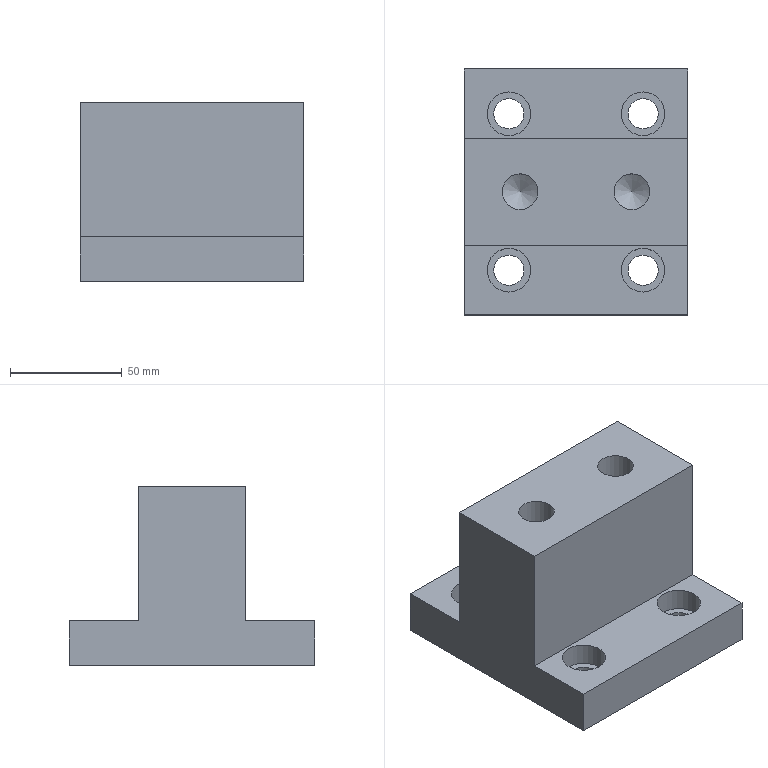Part | NX | features solid 2 | 1 solid | 26 faces | box 100 x 110 x 80 mm | volume 481642 mm3 | plane 14 | cylinder 10 | cone 2 | commonest cylinder face diameters 13.5 x4 19.5 x4 16 x2
STEP:
#1=CARTESIAN_POINT('',(-185.,-89.75,210.));
#2=VERTEX_POINT('',#1);
#3=CARTESIAN_POINT('',(-185.,-80.,210.));
#4=DIRECTION('',(0.,0.,-1.));
#5=DIRECTION('',(0.,-1.,0.));
#6=AXIS2_PLACEMENT_3D('',#3,#4,#5);
#7=CIRCLE('',#6,9.75);
#8=EDGE_CURVE('',#2,#2,#7,.T.);
#9=ORIENTED_EDGE('',*,*,#8,.T.);
#10=EDGE_LOOP('',(#9));
#11=FACE_BOUND('',#10,.T.);
#12=CARTESIAN_POINT('',(-245.,-89.75,210.));
#13=VERTEX_POINT('',#12);
#14=CARTESIAN_POINT('',(-245.,-80.,210.));
#15=DIRECTION('',(0.,0.,-1.));
#16=DIRECTION('',(0.,-1.,0.));
#17=AXIS2_PLACEMENT_3D('',#14,#15,#16);
#18=CIRCLE('',#17,9.75);
#19=EDGE_CURVE('',#13,#13,#18,.T.);
#20=ORIENTED_EDGE('',*,*,#19,.T.);
#21=EDGE_LOOP('',(#20));
#22=FACE_BOUND('',#21,.T.);
#23=CARTESIAN_POINT('',(-265.,-69.,210.));
#24=VERTEX_POINT('',#23);
#25=CARTESIAN_POINT('',(-165.,-69.,210.));
#26=VERTEX_POINT('',#25);
#27=CARTESIAN_POINT('',(-265.,-69.,210.));
#28=DIRECTION('',(1.,0.,0.));
#29=VECTOR('',#28,1000.);
#30=LINE('',#27,#29);
#31=EDGE_CURVE('',#24,#26,#30,.T.);
#32=ORIENTED_EDGE('',*,*,#31,.F.);
#33=CARTESIAN_POINT('',(-265.,-100.,210.));
#34=VERTEX_POINT('',#33);
#35=CARTESIAN_POINT('',(-265.,-100.,210.));
#36=DIRECTION('',(0.,-1.,0.));
#37=VECTOR('',#36,1000.);
#38=LINE('',#35,#37);
#39=EDGE_CURVE('',#34,#24,#38,.F.);
#40=ORIENTED_EDGE('',*,*,#39,.F.);
#41=CARTESIAN_POINT('',(-165.,-100.,210.));
#42=VERTEX_POINT('',#41);
#43=CARTESIAN_POINT('',(-265.,-100.,210.));
#44=DIRECTION('',(-1.,0.,0.));
#45=VECTOR('',#44,1000.);
#46=LINE('',#43,#45);
#47=EDGE_CURVE('',#34,#42,#46,.F.);
#48=ORIENTED_EDGE('',*,*,#47,.T.);
#49=CARTESIAN_POINT('',(-165.,-100.,210.));
#50=DIRECTION('',(0.,-1.,0.));
#51=VECTOR('',#50,1000.);
#52=LINE('',#49,#51);
#53=EDGE_CURVE('',#42,#26,#52,.F.);
#54=ORIENTED_EDGE('',*,*,#53,.T.);
#55=EDGE_LOOP('',(#32,#40,#48,#54));
#56=FACE_BOUND('',#55,.T.);
#57=CARTESIAN_POINT('',(-265.,-100.,210.));
#58=DIRECTION('',(0.,0.,-1.));
#59=DIRECTION('',(0.,-1.,0.));
#60=AXIS2_PLACEMENT_3D('',#57,#58,#59);
#61=PLANE('',#60);
#62=ADVANCED_FACE('',(#11,#22,#56),#61,.F.);
#63=CARTESIAN_POINT('',(-265.,-100.,190.));
#64=VERTEX_POINT('',#63);
#65=CARTESIAN_POINT('',(-265.,-100.,190.));
#66=DIRECTION('',(0.,0.,-1.));
#67=VECTOR('',#66,1000.);
#68=LINE('',#65,#67);
#69=EDGE_CURVE('',#64,#34,#68,.F.);
#70=ORIENTED_EDGE('',*,*,#69,.T.);
#71=ORIENTED_EDGE('',*,*,#39,.T.);
#72=CARTESIAN_POINT('',(-265.,-69.,270.));
#73=VERTEX_POINT('',#72);
#74=CARTESIAN_POINT('',(-265.,-69.,210.));
#75=DIRECTION('',(0.,0.,-1.));
#76=VECTOR('',#75,1000.);
#77=LINE('',#74,#76);
#78=EDGE_CURVE('',#24,#73,#77,.F.);
#79=ORIENTED_EDGE('',*,*,#78,.T.);
#80=CARTESIAN_POINT('',(-265.,-21.,270.));
#81=VERTEX_POINT('',#80);
#82=CARTESIAN_POINT('',(-265.,-69.,270.));
#83=DIRECTION('',(0.,-1.,0.));
#84=VECTOR('',#83,1000.);
#85=LINE('',#82,#84);
#86=EDGE_CURVE('',#73,#81,#85,.F.);
#87=ORIENTED_EDGE('',*,*,#86,.T.);
#88=CARTESIAN_POINT('',(-265.,-21.,210.));
#89=VERTEX_POINT('',#88);
#90=CARTESIAN_POINT('',(-265.,-21.,210.));
#91=DIRECTION('',(0.,0.,-1.));
#92=VECTOR('',#91,1000.);
#93=LINE('',#90,#92);
#94=EDGE_CURVE('',#89,#81,#93,.F.);
#95=ORIENTED_EDGE('',*,*,#94,.F.);
#96=CARTESIAN_POINT('',(-265.,10.,210.));
#97=VERTEX_POINT('',#96);
#98=CARTESIAN_POINT('',(-265.,-100.,210.));
#99=DIRECTION('',(0.,-1.,0.));
#100=VECTOR('',#99,1000.);
#101=LINE('',#98,#100);
#102=EDGE_CURVE('',#89,#97,#101,.F.);
#103=ORIENTED_EDGE('',*,*,#102,.T.);
#104=CARTESIAN_POINT('',(-265.,10.,190.));
#105=VERTEX_POINT('',#104);
#106=CARTESIAN_POINT('',(-265.,10.,190.));
#107=DIRECTION('',(0.,0.,-1.));
#108=VECTOR('',#107,1000.);
#109=LINE('',#106,#108);
#110=EDGE_CURVE('',#105,#97,#109,.F.);
#111=ORIENTED_EDGE('',*,*,#110,.F.);
#112=CARTESIAN_POINT('',(-265.,-100.,190.));
#113=DIRECTION('',(0.,1.,0.));
#114=VECTOR('',#113,1000.);
#115=LINE('',#112,#114);
#116=EDGE_CURVE('',#64,#105,#115,.T.);
#117=ORIENTED_EDGE('',*,*,#116,.F.);
#118=EDGE_LOOP('',(#70,#71,#79,#87,#95,#103,#111,#117));
#119=FACE_BOUND('',#118,.T.);
#120=CARTESIAN_POINT('',(-265.,-100.,190.));
#121=DIRECTION('',(-1.,0.,0.));
#122=DIRECTION('',(0.,1.,0.));
#123=AXIS2_PLACEMENT_3D('',#120,#121,#122);
#124=PLANE('',#123);
#125=ADVANCED_FACE('',(#119),#124,.T.);
#126=ORIENTED_EDGE('',*,*,#110,.T.);
#127=CARTESIAN_POINT('',(-165.,10.,210.));
#128=VERTEX_POINT('',#127);
#129=CARTESIAN_POINT('',(-265.,10.,210.));
#130=DIRECTION('',(-1.,0.,0.));
#131=VECTOR('',#130,1000.);
#132=LINE('',#129,#131);
#133=EDGE_CURVE('',#97,#128,#132,.F.);
#134=ORIENTED_EDGE('',*,*,#133,.T.);
#135=CARTESIAN_POINT('',(-165.,10.,190.));
#136=VERTEX_POINT('',#135);
#137=CARTESIAN_POINT('',(-165.,10.,190.));
#138=DIRECTION('',(0.,0.,-1.));
#139=VECTOR('',#138,1000.);
#140=LINE('',#137,#139);
#141=EDGE_CURVE('',#136,#128,#140,.F.);
#142=ORIENTED_EDGE('',*,*,#141,.F.);
#143=CARTESIAN_POINT('',(-265.,10.,190.));
#144=DIRECTION('',(1.,0.,0.));
#145=VECTOR('',#144,1000.);
#146=LINE('',#143,#145);
#147=EDGE_CURVE('',#105,#136,#146,.T.);
#148=ORIENTED_EDGE('',*,*,#147,.F.);
#149=EDGE_LOOP('',(#126,#134,#142,#148));
#150=FACE_BOUND('',#149,.T.);
#151=CARTESIAN_POINT('',(-265.,10.,190.));
#152=DIRECTION('',(0.,1.,0.));
#153=DIRECTION('',(1.,0.,0.));
#154=AXIS2_PLACEMENT_3D('',#151,#152,#153);
#155=PLANE('',#154);
#156=ADVANCED_FACE('',(#150),#155,.T.);
#157=ORIENTED_EDGE('',*,*,#141,.T.);
#158=CARTESIAN_POINT('',(-165.,-21.,210.));
#159=VERTEX_POINT('',#158);
#160=CARTESIAN_POINT('',(-165.,-100.,210.));
#161=DIRECTION('',(0.,-1.,0.));
#162=VECTOR('',#161,1000.);
#163=LINE('',#160,#162);
#164=EDGE_CURVE('',#159,#128,#163,.F.);
#165=ORIENTED_EDGE('',*,*,#164,.F.);
#166=CARTESIAN_POINT('',(-165.,-21.,270.));
#167=VERTEX_POINT('',#166);
#168=CARTESIAN_POINT('',(-165.,-21.,210.));
#169=DIRECTION('',(0.,0.,-1.));
#170=VECTOR('',#169,1000.);
#171=LINE('',#168,#170);
#172=EDGE_CURVE('',#159,#167,#171,.F.);
#173=ORIENTED_EDGE('',*,*,#172,.T.);
#174=CARTESIAN_POINT('',(-165.,-69.,270.));
#175=VERTEX_POINT('',#174);
#176=CARTESIAN_POINT('',(-165.,-69.,270.));
#177=DIRECTION('',(0.,-1.,0.));
#178=VECTOR('',#177,1000.);
#179=LINE('',#176,#178);
#180=EDGE_CURVE('',#175,#167,#179,.F.);
#181=ORIENTED_EDGE('',*,*,#180,.F.);
#182=CARTESIAN_POINT('',(-165.,-69.,210.));
#183=DIRECTION('',(0.,0.,-1.));
#184=VECTOR('',#183,1000.);
#185=LINE('',#182,#184);
#186=EDGE_CURVE('',#26,#175,#185,.F.);
#187=ORIENTED_EDGE('',*,*,#186,.F.);
#188=ORIENTED_EDGE('',*,*,#53,.F.);
#189=CARTESIAN_POINT('',(-165.,-100.,190.));
#190=VERTEX_POINT('',#189);
#191=CARTESIAN_POINT('',(-165.,-100.,190.));
#192=DIRECTION('',(0.,0.,-1.));
#193=VECTOR('',#192,1000.);
#194=LINE('',#191,#193);
#195=EDGE_CURVE('',#190,#42,#194,.F.);
#196=ORIENTED_EDGE('',*,*,#195,.F.);
#197=CARTESIAN_POINT('',(-165.,-100.,190.));
#198=DIRECTION('',(0.,1.,0.));
#199=VECTOR('',#198,1000.);
#200=LINE('',#197,#199);
#201=EDGE_CURVE('',#190,#136,#200,.T.);
#202=ORIENTED_EDGE('',*,*,#201,.T.);
#203=EDGE_LOOP('',(#157,#165,#173,#181,#187,#188,#196,#202));
#204=FACE_BOUND('',#203,.T.);
#205=CARTESIAN_POINT('',(-165.,-100.,190.));
#206=DIRECTION('',(-1.,0.,0.));
#207=DIRECTION('',(0.,1.,0.));
#208=AXIS2_PLACEMENT_3D('',#205,#206,#207);
#209=PLANE('',#208);
#210=ADVANCED_FACE('',(#204),#209,.F.);
#211=CARTESIAN_POINT('',(-265.,-100.,190.));
#212=DIRECTION('',(1.,0.,0.));
#213=VECTOR('',#212,1000.);
#214=LINE('',#211,#213);
#215=EDGE_CURVE('',#64,#190,#214,.T.);
#216=ORIENTED_EDGE('',*,*,#215,.T.);
#217=ORIENTED_EDGE('',*,*,#195,.T.);
#218=ORIENTED_EDGE('',*,*,#47,.F.);
#219=ORIENTED_EDGE('',*,*,#69,.F.);
#220=EDGE_LOOP('',(#216,#217,#218,#219));
#221=FACE_BOUND('',#220,.T.);
#222=CARTESIAN_POINT('',(-265.,-100.,190.));
#223=DIRECTION('',(0.,1.,0.));
#224=DIRECTION('',(1.,0.,0.));
#225=AXIS2_PLACEMENT_3D('',#222,#223,#224);
#226=PLANE('',#225);
#227=ADVANCED_FACE('',(#221),#226,.F.);
#228=CARTESIAN_POINT('',(-185.,-19.75,210.));
#229=VERTEX_POINT('',#228);
#230=CARTESIAN_POINT('',(-185.,-10.,210.));
#231=DIRECTION('',(0.,0.,-1.));
#232=DIRECTION('',(0.,-1.,0.));
#233=AXIS2_PLACEMENT_3D('',#230,#231,#232);
#234=CIRCLE('',#233,9.75);
#235=EDGE_CURVE('',#229,#229,#234,.T.);
#236=ORIENTED_EDGE('',*,*,#235,.T.);
#237=EDGE_LOOP('',(#236));
#238=FACE_BOUND('',#237,.T.);
#239=CARTESIAN_POINT('',(-245.,-19.75,210.));
#240=VERTEX_POINT('',#239);
#241=CARTESIAN_POINT('',(-245.,-10.,210.));
#242=DIRECTION('',(0.,0.,-1.));
#243=DIRECTION('',(0.,-1.,0.));
#244=AXIS2_PLACEMENT_3D('',#241,#242,#243);
#245=CIRCLE('',#244,9.75);
#246=EDGE_CURVE('',#240,#240,#245,.T.);
#247=ORIENTED_EDGE('',*,*,#246,.T.);
#248=EDGE_LOOP('',(#247));
#249=FACE_BOUND('',#248,.T.);
#250=ORIENTED_EDGE('',*,*,#102,.F.);
#251=CARTESIAN_POINT('',(-265.,-21.,210.));
#252=DIRECTION('',(1.,0.,0.));
#253=VECTOR('',#252,1000.);
#254=LINE('',#251,#253);
#255=EDGE_CURVE('',#89,#159,#254,.T.);
#256=ORIENTED_EDGE('',*,*,#255,.T.);
#257=ORIENTED_EDGE('',*,*,#164,.T.);
#258=ORIENTED_EDGE('',*,*,#133,.F.);
#259=EDGE_LOOP('',(#250,#256,#257,#258));
#260=FACE_BOUND('',#259,.T.);
#261=CARTESIAN_POINT('',(-265.,-100.,210.));
#262=DIRECTION('',(0.,0.,-1.));
#263=DIRECTION('',(0.,-1.,0.));
#264=AXIS2_PLACEMENT_3D('',#261,#262,#263);
#265=PLANE('',#264);
#266=ADVANCED_FACE('',(#238,#249,#260),#265,.F.);
#267=CARTESIAN_POINT('',(-185.,-16.75,190.));
#268=VERTEX_POINT('',#267);
#269=CARTESIAN_POINT('',(-185.,-10.,190.));
#270=DIRECTION('',(0.,0.,-1.));
#271=DIRECTION('',(0.,-1.,0.));
#272=AXIS2_PLACEMENT_3D('',#269,#270,#271);
#273=CIRCLE('',#272,6.75);
#274=EDGE_CURVE('',#268,#268,#273,.T.);
#275=ORIENTED_EDGE('',*,*,#274,.F.);
#276=EDGE_LOOP('',(#275));
#277=FACE_BOUND('',#276,.T.);
#278=CARTESIAN_POINT('',(-245.,-16.75,190.));
#279=VERTEX_POINT('',#278);
#280=CARTESIAN_POINT('',(-245.,-10.,190.));
#281=DIRECTION('',(0.,0.,-1.));
#282=DIRECTION('',(0.,-1.,0.));
#283=AXIS2_PLACEMENT_3D('',#280,#281,#282);
#284=CIRCLE('',#283,6.75);
#285=EDGE_CURVE('',#279,#279,#284,.T.);
#286=ORIENTED_EDGE('',*,*,#285,.F.);
#287=EDGE_LOOP('',(#286));
#288=FACE_BOUND('',#287,.T.);
#289=CARTESIAN_POINT('',(-185.,-86.75,190.));
#290=VERTEX_POINT('',#289);
#291=CARTESIAN_POINT('',(-185.,-80.,190.));
#292=DIRECTION('',(0.,0.,-1.));
#293=DIRECTION('',(0.,-1.,0.));
#294=AXIS2_PLACEMENT_3D('',#291,#292,#293);
#295=CIRCLE('',#294,6.75);
#296=EDGE_CURVE('',#290,#290,#295,.T.);
#297=ORIENTED_EDGE('',*,*,#296,.F.);
#298=EDGE_LOOP('',(#297));
#299=FACE_BOUND('',#298,.T.);
#300=CARTESIAN_POINT('',(-245.,-86.75,190.));
#301=VERTEX_POINT('',#300);
#302=CARTESIAN_POINT('',(-245.,-80.,190.));
#303=DIRECTION('',(0.,0.,-1.));
#304=DIRECTION('',(0.,-1.,0.));
#305=AXIS2_PLACEMENT_3D('',#302,#303,#304);
#306=CIRCLE('',#305,6.75);
#307=EDGE_CURVE('',#301,#301,#306,.T.);
#308=ORIENTED_EDGE('',*,*,#307,.F.);
#309=EDGE_LOOP('',(#308));
#310=FACE_BOUND('',#309,.T.);
#311=ORIENTED_EDGE('',*,*,#201,.F.);
#312=ORIENTED_EDGE('',*,*,#215,.F.);
#313=ORIENTED_EDGE('',*,*,#116,.T.);
#314=ORIENTED_EDGE('',*,*,#147,.T.);
#315=EDGE_LOOP('',(#311,#312,#313,#314));
#316=FACE_BOUND('',#315,.T.);
#317=CARTESIAN_POINT('',(-265.,-100.,190.));
#318=DIRECTION('',(0.,0.,-1.));
#319=DIRECTION('',(0.,-1.,0.));
#320=AXIS2_PLACEMENT_3D('',#317,#318,#319);
#321=PLANE('',#320);
#322=ADVANCED_FACE('',(#277,#288,#299,#310,#316),#321,.T.);
#323=ORIENTED_EDGE('',*,*,#94,.T.);
#324=CARTESIAN_POINT('',(-265.,-21.,270.));
#325=DIRECTION('',(-1.,0.,0.));
#326=VECTOR('',#325,1000.);
#327=LINE('',#324,#326);
#328=EDGE_CURVE('',#81,#167,#327,.F.);
#329=ORIENTED_EDGE('',*,*,#328,.T.);
#330=ORIENTED_EDGE('',*,*,#172,.F.);
#331=ORIENTED_EDGE('',*,*,#255,.F.);
#332=EDGE_LOOP('',(#323,#329,#330,#331));
#333=FACE_BOUND('',#332,.T.);
#334=CARTESIAN_POINT('',(-265.,-21.,210.));
#335=DIRECTION('',(0.,1.,0.));
#336=DIRECTION('',(1.,0.,0.));
#337=AXIS2_PLACEMENT_3D('',#334,#335,#336);
#338=PLANE('',#337);
#339=ADVANCED_FACE('',(#333),#338,.T.);
#340=ORIENTED_EDGE('',*,*,#31,.T.);
#341=ORIENTED_EDGE('',*,*,#186,.T.);
#342=CARTESIAN_POINT('',(-265.,-69.,270.));
#343=DIRECTION('',(-1.,0.,0.));
#344=VECTOR('',#343,1000.);
#345=LINE('',#342,#344);
#346=EDGE_CURVE('',#73,#175,#345,.F.);
#347=ORIENTED_EDGE('',*,*,#346,.F.);
#348=ORIENTED_EDGE('',*,*,#78,.F.);
#349=EDGE_LOOP('',(#340,#341,#347,#348));
#350=FACE_BOUND('',#349,.T.);
#351=CARTESIAN_POINT('',(-265.,-69.,210.));
#352=DIRECTION('',(0.,1.,0.));
#353=DIRECTION('',(1.,0.,0.));
#354=AXIS2_PLACEMENT_3D('',#351,#352,#353);
#355=PLANE('',#354);
#356=ADVANCED_FACE('',(#350),#355,.F.);
#357=CARTESIAN_POINT('',(-190.,-53.,270.));
#358=VERTEX_POINT('',#357);
#359=CARTESIAN_POINT('',(-190.,-45.,270.));
#360=DIRECTION('',(0.,0.,-1.));
#361=DIRECTION('',(0.,-1.,0.));
#362=AXIS2_PLACEMENT_3D('',#359,#360,#361);
#363=CIRCLE('',#362,8.);
#364=EDGE_CURVE('',#358,#358,#363,.T.);
#365=ORIENTED_EDGE('',*,*,#364,.T.);
#366=EDGE_LOOP('',(#365));
#367=FACE_BOUND('',#366,.T.);
#368=CARTESIAN_POINT('',(-240.,-53.,270.));
#369=VERTEX_POINT('',#368);
#370=CARTESIAN_POINT('',(-240.,-45.,270.));
#371=DIRECTION('',(0.,0.,-1.));
#372=DIRECTION('',(0.,-1.,0.));
#373=AXIS2_PLACEMENT_3D('',#370,#371,#372);
#374=CIRCLE('',#373,8.);
#375=EDGE_CURVE('',#369,#369,#374,.T.);
#376=ORIENTED_EDGE('',*,*,#375,.T.);
#377=EDGE_LOOP('',(#376));
#378=FACE_BOUND('',#377,.T.);
#379=ORIENTED_EDGE('',*,*,#180,.T.);
#380=ORIENTED_EDGE('',*,*,#328,.F.);
#381=ORIENTED_EDGE('',*,*,#86,.F.);
#382=ORIENTED_EDGE('',*,*,#346,.T.);
#383=EDGE_LOOP('',(#379,#380,#381,#382));
#384=FACE_BOUND('',#383,.T.);
#385=CARTESIAN_POINT('',(-265.,-69.,270.));
#386=DIRECTION('',(0.,0.,-1.));
#387=DIRECTION('',(0.,-1.,0.));
#388=AXIS2_PLACEMENT_3D('',#385,#386,#387);
#389=PLANE('',#388);
#390=ADVANCED_FACE('',(#367,#378,#384),#389,.F.);
#391=ORIENTED_EDGE('',*,*,#307,.T.);
#392=EDGE_LOOP('',(#391));
#393=FACE_BOUND('',#392,.T.);
#394=CARTESIAN_POINT('',(-245.,-86.75,200.));
#395=VERTEX_POINT('',#394);
#396=CARTESIAN_POINT('',(-245.,-80.,200.));
#397=DIRECTION('',(0.,0.,-1.));
#398=DIRECTION('',(0.,-1.,0.));
#399=AXIS2_PLACEMENT_3D('',#396,#397,#398);
#400=CIRCLE('',#399,6.75);
#401=EDGE_CURVE('',#395,#395,#400,.T.);
#402=ORIENTED_EDGE('',*,*,#401,.F.);
#403=EDGE_LOOP('',(#402));
#404=FACE_BOUND('',#403,.T.);
#405=CARTESIAN_POINT('',(-245.,-80.,160.));
#406=DIRECTION('',(0.,0.,-1.));
#407=DIRECTION('',(0.,-1.,0.));
#408=AXIS2_PLACEMENT_3D('',#405,#406,#407);
#409=CYLINDRICAL_SURFACE('',#408,6.75);
#410=ADVANCED_FACE('',(#393,#404),#409,.F.);
#411=ORIENTED_EDGE('',*,*,#401,.T.);
#412=EDGE_LOOP('',(#411));
#413=FACE_BOUND('',#412,.T.);
#414=CARTESIAN_POINT('',(-245.,-89.75,200.));
#415=VERTEX_POINT('',#414);
#416=CARTESIAN_POINT('',(-245.,-80.,200.));
#417=DIRECTION('',(0.,0.,-1.));
#418=DIRECTION('',(0.,-1.,0.));
#419=AXIS2_PLACEMENT_3D('',#416,#417,#418);
#420=CIRCLE('',#419,9.75);
#421=EDGE_CURVE('',#415,#415,#420,.T.);
#422=ORIENTED_EDGE('',*,*,#421,.F.);
#423=EDGE_LOOP('',(#422));
#424=FACE_BOUND('',#423,.T.);
#425=CARTESIAN_POINT('',(-245.,-80.,200.));
#426=DIRECTION('',(0.,0.,-1.));
#427=DIRECTION('',(0.,-1.,0.));
#428=AXIS2_PLACEMENT_3D('',#425,#426,#427);
#429=PLANE('',#428);
#430=ADVANCED_FACE('',(#413,#424),#429,.F.);
#431=ORIENTED_EDGE('',*,*,#421,.T.);
#432=EDGE_LOOP('',(#431));
#433=FACE_BOUND('',#432,.T.);
#434=ORIENTED_EDGE('',*,*,#19,.F.);
#435=EDGE_LOOP('',(#434));
#436=FACE_BOUND('',#435,.T.);
#437=CARTESIAN_POINT('',(-245.,-80.,210.));
#438=DIRECTION('',(0.,0.,-1.));
#439=DIRECTION('',(0.,-1.,0.));
#440=AXIS2_PLACEMENT_3D('',#437,#438,#439);
#441=CYLINDRICAL_SURFACE('',#440,9.75);
#442=ADVANCED_FACE('',(#433,#436),#441,.F.);
#443=ORIENTED_EDGE('',*,*,#296,.T.);
#444=EDGE_LOOP('',(#443));
#445=FACE_BOUND('',#444,.T.);
#446=CARTESIAN_POINT('',(-185.,-86.75,200.));
#447=VERTEX_POINT('',#446);
#448=CARTESIAN_POINT('',(-185.,-80.,200.));
#449=DIRECTION('',(0.,0.,-1.));
#450=DIRECTION('',(0.,-1.,0.));
#451=AXIS2_PLACEMENT_3D('',#448,#449,#450);
#452=CIRCLE('',#451,6.75);
#453=EDGE_CURVE('',#447,#447,#452,.T.);
#454=ORIENTED_EDGE('',*,*,#453,.F.);
#455=EDGE_LOOP('',(#454));
#456=FACE_BOUND('',#455,.T.);
#457=CARTESIAN_POINT('',(-185.,-80.,160.));
#458=DIRECTION('',(0.,0.,-1.));
#459=DIRECTION('',(0.,-1.,0.));
#460=AXIS2_PLACEMENT_3D('',#457,#458,#459);
#461=CYLINDRICAL_SURFACE('',#460,6.75);
#462=ADVANCED_FACE('',(#445,#456),#461,.F.);
#463=ORIENTED_EDGE('',*,*,#453,.T.);
#464=EDGE_LOOP('',(#463));
#465=FACE_BOUND('',#464,.T.);
#466=CARTESIAN_POINT('',(-185.,-89.75,200.));
#467=VERTEX_POINT('',#466);
#468=CARTESIAN_POINT('',(-185.,-80.,200.));
#469=DIRECTION('',(0.,0.,-1.));
#470=DIRECTION('',(0.,-1.,0.));
#471=AXIS2_PLACEMENT_3D('',#468,#469,#470);
#472=CIRCLE('',#471,9.75);
#473=EDGE_CURVE('',#467,#467,#472,.T.);
#474=ORIENTED_EDGE('',*,*,#473,.F.);
#475=EDGE_LOOP('',(#474));
#476=FACE_BOUND('',#475,.T.);
#477=CARTESIAN_POINT('',(-185.,-80.,200.));
#478=DIRECTION('',(0.,0.,-1.));
#479=DIRECTION('',(0.,-1.,0.));
#480=AXIS2_PLACEMENT_3D('',#477,#478,#479);
#481=PLANE('',#480);
#482=ADVANCED_FACE('',(#465,#476),#481,.F.);
#483=ORIENTED_EDGE('',*,*,#473,.T.);
#484=EDGE_LOOP('',(#483));
#485=FACE_BOUND('',#484,.T.);
#486=ORIENTED_EDGE('',*,*,#8,.F.);
#487=EDGE_LOOP('',(#486));
#488=FACE_BOUND('',#487,.T.);
#489=CARTESIAN_POINT('',(-185.,-80.,210.));
#490=DIRECTION('',(0.,0.,-1.));
#491=DIRECTION('',(0.,-1.,0.));
#492=AXIS2_PLACEMENT_3D('',#489,#490,#491);
#493=CYLINDRICAL_SURFACE('',#492,9.75);
#494=ADVANCED_FACE('',(#485,#488),#493,.F.);
#495=ORIENTED_EDGE('',*,*,#285,.T.);
#496=EDGE_LOOP('',(#495));
#497=FACE_BOUND('',#496,.T.);
#498=CARTESIAN_POINT('',(-245.,-16.75,200.));
#499=VERTEX_POINT('',#498);
#500=CARTESIAN_POINT('',(-245.,-10.,200.));
#501=DIRECTION('',(0.,0.,-1.));
#502=DIRECTION('',(0.,-1.,0.));
#503=AXIS2_PLACEMENT_3D('',#500,#501,#502);
#504=CIRCLE('',#503,6.75);
#505=EDGE_CURVE('',#499,#499,#504,.T.);
#506=ORIENTED_EDGE('',*,*,#505,.F.);
#507=EDGE_LOOP('',(#506));
#508=FACE_BOUND('',#507,.T.);
#509=CARTESIAN_POINT('',(-245.,-10.,160.));
#510=DIRECTION('',(0.,0.,-1.));
#511=DIRECTION('',(0.,-1.,0.));
#512=AXIS2_PLACEMENT_3D('',#509,#510,#511);
#513=CYLINDRICAL_SURFACE('',#512,6.75);
#514=ADVANCED_FACE('',(#497,#508),#513,.F.);
#515=ORIENTED_EDGE('',*,*,#505,.T.);
#516=EDGE_LOOP('',(#515));
#517=FACE_BOUND('',#516,.T.);
#518=CARTESIAN_POINT('',(-245.,-19.75,200.));
#519=VERTEX_POINT('',#518);
#520=CARTESIAN_POINT('',(-245.,-10.,200.));
#521=DIRECTION('',(0.,0.,-1.));
#522=DIRECTION('',(0.,-1.,0.));
#523=AXIS2_PLACEMENT_3D('',#520,#521,#522);
#524=CIRCLE('',#523,9.75);
#525=EDGE_CURVE('',#519,#519,#524,.T.);
#526=ORIENTED_EDGE('',*,*,#525,.F.);
#527=EDGE_LOOP('',(#526));
#528=FACE_BOUND('',#527,.T.);
#529=CARTESIAN_POINT('',(-245.,-10.,200.));
#530=DIRECTION('',(0.,0.,-1.));
#531=DIRECTION('',(0.,-1.,0.));
#532=AXIS2_PLACEMENT_3D('',#529,#530,#531);
#533=PLANE('',#532);
#534=ADVANCED_FACE('',(#517,#528),#533,.F.);
#535=ORIENTED_EDGE('',*,*,#525,.T.);
#536=EDGE_LOOP('',(#535));
#537=FACE_BOUND('',#536,.T.);
#538=ORIENTED_EDGE('',*,*,#246,.F.);
#539=EDGE_LOOP('',(#538));
#540=FACE_BOUND('',#539,.T.);
#541=CARTESIAN_POINT('',(-245.,-10.,210.));
#542=DIRECTION('',(0.,0.,-1.));
#543=DIRECTION('',(0.,-1.,0.));
#544=AXIS2_PLACEMENT_3D('',#541,#542,#543);
#545=CYLINDRICAL_SURFACE('',#544,9.75);
#546=ADVANCED_FACE('',(#537,#540),#545,.F.);
#547=ORIENTED_EDGE('',*,*,#274,.T.);
#548=EDGE_LOOP('',(#547));
#549=FACE_BOUND('',#548,.T.);
#550=CARTESIAN_POINT('',(-185.,-16.75,200.));
#551=VERTEX_POINT('',#550);
#552=CARTESIAN_POINT('',(-185.,-10.,200.));
#553=DIRECTION('',(0.,0.,-1.));
#554=DIRECTION('',(0.,-1.,0.));
#555=AXIS2_PLACEMENT_3D('',#552,#553,#554);
#556=CIRCLE('',#555,6.75);
#557=EDGE_CURVE('',#551,#551,#556,.T.);
#558=ORIENTED_EDGE('',*,*,#557,.F.);
#559=EDGE_LOOP('',(#558));
#560=FACE_BOUND('',#559,.T.);
#561=CARTESIAN_POINT('',(-185.,-10.,160.));
#562=DIRECTION('',(0.,0.,-1.));
#563=DIRECTION('',(0.,-1.,0.));
#564=AXIS2_PLACEMENT_3D('',#561,#562,#563);
#565=CYLINDRICAL_SURFACE('',#564,6.75);
#566=ADVANCED_FACE('',(#549,#560),#565,.F.);
#567=ORIENTED_EDGE('',*,*,#557,.T.);
#568=EDGE_LOOP('',(#567));
#569=FACE_BOUND('',#568,.T.);
#570=CARTESIAN_POINT('',(-185.,-19.75,200.));
#571=VERTEX_POINT('',#570);
#572=CARTESIAN_POINT('',(-185.,-10.,200.));
#573=DIRECTION('',(0.,0.,-1.));
#574=DIRECTION('',(0.,-1.,0.));
#575=AXIS2_PLACEMENT_3D('',#572,#573,#574);
#576=CIRCLE('',#575,9.75);
#577=EDGE_CURVE('',#571,#571,#576,.T.);
#578=ORIENTED_EDGE('',*,*,#577,.F.);
#579=EDGE_LOOP('',(#578));
#580=FACE_BOUND('',#579,.T.);
#581=CARTESIAN_POINT('',(-185.,-10.,200.));
#582=DIRECTION('',(0.,0.,-1.));
#583=DIRECTION('',(0.,-1.,0.));
#584=AXIS2_PLACEMENT_3D('',#581,#582,#583);
#585=PLANE('',#584);
#586=ADVANCED_FACE('',(#569,#580),#585,.F.);
#587=ORIENTED_EDGE('',*,*,#577,.T.);
#588=EDGE_LOOP('',(#587));
#589=FACE_BOUND('',#588,.T.);
#590=ORIENTED_EDGE('',*,*,#235,.F.);
#591=EDGE_LOOP('',(#590));
#592=FACE_BOUND('',#591,.T.);
#593=CARTESIAN_POINT('',(-185.,-10.,210.));
#594=DIRECTION('',(0.,0.,-1.));
#595=DIRECTION('',(0.,-1.,0.));
#596=AXIS2_PLACEMENT_3D('',#593,#594,#595);
#597=CYLINDRICAL_SURFACE('',#596,9.75);
#598=ADVANCED_FACE('',(#589,#592),#597,.F.);
#599=CARTESIAN_POINT('',(-240.,-53.,250.));
#600=VERTEX_POINT('',#599);
#601=CARTESIAN_POINT('',(-240.,-45.,250.));
#602=DIRECTION('',(0.,0.,-1.));
#603=DIRECTION('',(0.,-1.,0.));
#604=AXIS2_PLACEMENT_3D('',#601,#602,#603);
#605=CIRCLE('',#604,8.);
#606=EDGE_CURVE('',#600,#600,#605,.T.);
#607=ORIENTED_EDGE('',*,*,#606,.F.);
#608=EDGE_LOOP('',(#607));
#609=FACE_BOUND('',#608,.T.);
#610=CARTESIAN_POINT('',(-240.,-45.,245.193));
#611=VERTEX_POINT('',#610);
#612=VERTEX_LOOP('',#611);
#613=FACE_BOUND('',#612,.T.);
#614=CARTESIAN_POINT('',(-240.,-45.,250.));
#615=DIRECTION('',(0.,0.,1.));
#616=DIRECTION('',(0.,1.,0.));
#617=AXIS2_PLACEMENT_3D('',#614,#615,#616);
#618=CONICAL_SURFACE('',#617,8.,1.03);
#619=ADVANCED_FACE('',(#609,#613),#618,.F.);
#620=ORIENTED_EDGE('',*,*,#606,.T.);
#621=EDGE_LOOP('',(#620));
#622=FACE_BOUND('',#621,.T.);
#623=ORIENTED_EDGE('',*,*,#375,.F.);
#624=EDGE_LOOP('',(#623));
#625=FACE_BOUND('',#624,.T.);
#626=CARTESIAN_POINT('',(-240.,-45.,270.));
#627=DIRECTION('',(0.,0.,-1.));
#628=DIRECTION('',(0.,-1.,0.));
#629=AXIS2_PLACEMENT_3D('',#626,#627,#628);
#630=CYLINDRICAL_SURFACE('',#629,8.);
#631=ADVANCED_FACE('',(#622,#625),#630,.F.);
#632=CARTESIAN_POINT('',(-190.,-53.,250.));
#633=VERTEX_POINT('',#632);
#634=CARTESIAN_POINT('',(-190.,-45.,250.));
#635=DIRECTION('',(0.,0.,-1.));
#636=DIRECTION('',(0.,-1.,0.));
#637=AXIS2_PLACEMENT_3D('',#634,#635,#636);
#638=CIRCLE('',#637,8.);
#639=EDGE_CURVE('',#633,#633,#638,.T.);
#640=ORIENTED_EDGE('',*,*,#639,.F.);
#641=EDGE_LOOP('',(#640));
#642=FACE_BOUND('',#641,.T.);
#643=CARTESIAN_POINT('',(-190.,-45.,245.193));
#644=VERTEX_POINT('',#643);
#645=VERTEX_LOOP('',#644);
#646=FACE_BOUND('',#645,.T.);
#647=CARTESIAN_POINT('',(-190.,-45.,250.));
#648=DIRECTION('',(0.,0.,1.));
#649=DIRECTION('',(0.,1.,0.));
#650=AXIS2_PLACEMENT_3D('',#647,#648,#649);
#651=CONICAL_SURFACE('',#650,8.,1.03);
#652=ADVANCED_FACE('',(#642,#646),#651,.F.);
#653=ORIENTED_EDGE('',*,*,#639,.T.);
#654=EDGE_LOOP('',(#653));
#655=FACE_BOUND('',#654,.T.);
#656=ORIENTED_EDGE('',*,*,#364,.F.);
#657=EDGE_LOOP('',(#656));
#658=FACE_BOUND('',#657,.T.);
#659=CARTESIAN_POINT('',(-190.,-45.,270.));
#660=DIRECTION('',(0.,0.,-1.));
#661=DIRECTION('',(0.,-1.,0.));
#662=AXIS2_PLACEMENT_3D('',#659,#660,#661);
#663=CYLINDRICAL_SURFACE('',#662,8.);
#664=ADVANCED_FACE('',(#655,#658),#663,.F.);
#665=CLOSED_SHELL('',(#62,#125,#156,#210,#227,#266,#322,#339,#356,#390,#410,#430,#442,#462,#482,#494,#514,#534,#546,#566,#586,#598,#619,#631,#652,#664));
#666=MANIFOLD_SOLID_BREP('',#665);
#667=(LENGTH_UNIT()NAMED_UNIT(*)SI_UNIT(.MILLI.,.METRE.));
#668=UNCERTAINTY_MEASURE_WITH_UNIT(LENGTH_MEASURE(0.00001),#667,'','');
#669=(NAMED_UNIT(*)PLANE_ANGLE_UNIT()SI_UNIT($,.RADIAN.));
#670=(NAMED_UNIT(*)SI_UNIT($,.STERADIAN.)SOLID_ANGLE_UNIT());
#671=(GEOMETRIC_REPRESENTATION_CONTEXT(3)GLOBAL_UNCERTAINTY_ASSIGNED_CONTEXT((#668))GLOBAL_UNIT_ASSIGNED_CONTEXT((#667,#669,#670))REPRESENTATION_CONTEXT('',''));
#672=ADVANCED_BREP_SHAPE_REPRESENTATION('',(#666),#671);